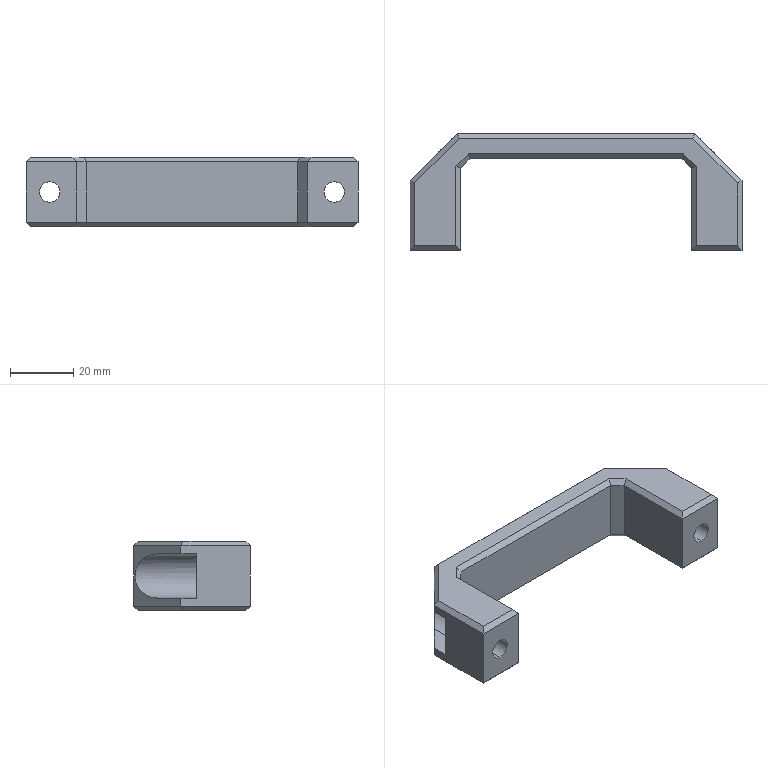Part | SolidWorks | features Chamfer 1, Extrusion 1, HoleWzd 1, ICE 1 | 1 solid | 56 faces | box 105 x 37 x 22 mm | volume 26847 mm3 | plane 46 | cylinder 10 | commonest cylinder face diameters 6.5 x4 11 x4 14 x2
STEP:
#1=CARTESIAN_POINT('',(-45.,0.,-3.25));
#2=VERTEX_POINT('',#1);
#3=CARTESIAN_POINT('',(-45.,0.,3.25));
#4=VERTEX_POINT('',#3);
#5=CARTESIAN_POINT('',(-45.,0.,0.));
#6=DIRECTION('',(0.,1.,0.));
#7=DIRECTION('',(0.,0.,1.));
#8=AXIS2_PLACEMENT_3D('',#5,#6,#7);
#9=CIRCLE('',#8,3.25);
#10=EDGE_CURVE('',#2,#4,#9,.T.);
#11=ORIENTED_EDGE('',*,*,#10,.F.);
#12=CARTESIAN_POINT('',(-45.,7.,-3.25));
#13=VERTEX_POINT('',#12);
#14=CARTESIAN_POINT('',(-45.,37.,-3.25));
#15=DIRECTION('',(0.,1.,0.));
#16=VECTOR('',#15,1000.);
#17=LINE('',#14,#16);
#18=EDGE_CURVE('',#2,#13,#17,.T.);
#19=ORIENTED_EDGE('',*,*,#18,.T.);
#20=CARTESIAN_POINT('',(-45.,7.,3.25));
#21=VERTEX_POINT('',#20);
#22=CARTESIAN_POINT('',(-45.,7.,0.));
#23=DIRECTION('',(0.,1.,0.));
#24=DIRECTION('',(0.,0.,1.));
#25=AXIS2_PLACEMENT_3D('',#22,#23,#24);
#26=CIRCLE('',#25,3.25);
#27=EDGE_CURVE('',#13,#21,#26,.T.);
#28=ORIENTED_EDGE('',*,*,#27,.T.);
#29=CARTESIAN_POINT('',(-45.,37.,3.25));
#30=DIRECTION('',(0.,1.,0.));
#31=VECTOR('',#30,1000.);
#32=LINE('',#29,#31);
#33=EDGE_CURVE('',#4,#21,#32,.T.);
#34=ORIENTED_EDGE('',*,*,#33,.F.);
#35=EDGE_LOOP('',(#11,#19,#28,#34));
#36=FACE_OUTER_BOUND('',#35,.T.);
#37=CARTESIAN_POINT('',(-45.,37.,0.));
#38=DIRECTION('',(0.,1.,0.));
#39=DIRECTION('',(0.,0.,1.));
#40=AXIS2_PLACEMENT_3D('',#37,#38,#39);
#41=CYLINDRICAL_SURFACE('',#40,3.25);
#42=ADVANCED_FACE('',(#36),#41,.F.);
#43=CARTESIAN_POINT('',(45.,0.,-3.25));
#44=VERTEX_POINT('',#43);
#45=CARTESIAN_POINT('',(45.,0.,3.25));
#46=VERTEX_POINT('',#45);
#47=CARTESIAN_POINT('',(45.,0.,0.));
#48=DIRECTION('',(0.,1.,0.));
#49=DIRECTION('',(0.,0.,1.));
#50=AXIS2_PLACEMENT_3D('',#47,#48,#49);
#51=CIRCLE('',#50,3.25);
#52=EDGE_CURVE('',#44,#46,#51,.T.);
#53=ORIENTED_EDGE('',*,*,#52,.F.);
#54=CARTESIAN_POINT('',(45.,7.,-3.25));
#55=VERTEX_POINT('',#54);
#56=CARTESIAN_POINT('',(45.,37.,-3.25));
#57=DIRECTION('',(0.,1.,0.));
#58=VECTOR('',#57,1000.);
#59=LINE('',#56,#58);
#60=EDGE_CURVE('',#44,#55,#59,.T.);
#61=ORIENTED_EDGE('',*,*,#60,.T.);
#62=CARTESIAN_POINT('',(45.,7.,3.25));
#63=VERTEX_POINT('',#62);
#64=CARTESIAN_POINT('',(45.,7.,0.));
#65=DIRECTION('',(0.,1.,0.));
#66=DIRECTION('',(0.,0.,1.));
#67=AXIS2_PLACEMENT_3D('',#64,#65,#66);
#68=CIRCLE('',#67,3.25);
#69=EDGE_CURVE('',#55,#63,#68,.T.);
#70=ORIENTED_EDGE('',*,*,#69,.T.);
#71=CARTESIAN_POINT('',(45.,37.,3.25));
#72=DIRECTION('',(0.,1.,0.));
#73=VECTOR('',#72,1000.);
#74=LINE('',#71,#73);
#75=EDGE_CURVE('',#46,#63,#74,.T.);
#76=ORIENTED_EDGE('',*,*,#75,.F.);
#77=EDGE_LOOP('',(#53,#61,#70,#76));
#78=FACE_OUTER_BOUND('',#77,.T.);
#79=CARTESIAN_POINT('',(45.,37.,0.));
#80=DIRECTION('',(0.,1.,0.));
#81=DIRECTION('',(0.,0.,1.));
#82=AXIS2_PLACEMENT_3D('',#79,#80,#81);
#83=CYLINDRICAL_SURFACE('',#82,3.25);
#84=ADVANCED_FACE('',(#78),#83,.F.);
#85=CARTESIAN_POINT('',(45.,7.,-5.5));
#86=VERTEX_POINT('',#85);
#87=CARTESIAN_POINT('',(45.,7.,5.5));
#88=VERTEX_POINT('',#87);
#89=CARTESIAN_POINT('',(45.,7.,0.));
#90=DIRECTION('',(0.,1.,0.));
#91=DIRECTION('',(0.,0.,1.));
#92=AXIS2_PLACEMENT_3D('',#89,#90,#91);
#93=CIRCLE('',#92,5.5);
#94=EDGE_CURVE('',#86,#88,#93,.T.);
#95=ORIENTED_EDGE('',*,*,#94,.F.);
#96=CARTESIAN_POINT('',(45.,17.,-5.5));
#97=VERTEX_POINT('',#96);
#98=CARTESIAN_POINT('',(45.,37.,-5.5));
#99=DIRECTION('',(0.,1.,0.));
#100=VECTOR('',#99,1000.);
#101=LINE('',#98,#100);
#102=EDGE_CURVE('',#86,#97,#101,.T.);
#103=ORIENTED_EDGE('',*,*,#102,.T.);
#104=CARTESIAN_POINT('',(45.,17.,5.5));
#105=VERTEX_POINT('',#104);
#106=CARTESIAN_POINT('',(45.,17.,0.));
#107=DIRECTION('',(0.,1.,0.));
#108=DIRECTION('',(0.,0.,-1.));
#109=AXIS2_PLACEMENT_3D('',#106,#107,#108);
#110=CIRCLE('',#109,5.5);
#111=EDGE_CURVE('',#97,#105,#110,.T.);
#112=ORIENTED_EDGE('',*,*,#111,.T.);
#113=CARTESIAN_POINT('',(45.,37.,5.5));
#114=DIRECTION('',(0.,1.,0.));
#115=VECTOR('',#114,1000.);
#116=LINE('',#113,#115);
#117=EDGE_CURVE('',#88,#105,#116,.T.);
#118=ORIENTED_EDGE('',*,*,#117,.F.);
#119=EDGE_LOOP('',(#95,#103,#112,#118));
#120=FACE_OUTER_BOUND('',#119,.T.);
#121=CARTESIAN_POINT('',(45.,37.,0.));
#122=DIRECTION('',(0.,1.,0.));
#123=DIRECTION('',(0.,0.,1.));
#124=AXIS2_PLACEMENT_3D('',#121,#122,#123);
#125=CYLINDRICAL_SURFACE('',#124,5.5);
#126=ADVANCED_FACE('',(#120),#125,.F.);
#127=CARTESIAN_POINT('',(-45.,7.,-5.5));
#128=VERTEX_POINT('',#127);
#129=CARTESIAN_POINT('',(-45.,7.,5.5));
#130=VERTEX_POINT('',#129);
#131=CARTESIAN_POINT('',(-45.,7.,0.));
#132=DIRECTION('',(0.,1.,0.));
#133=DIRECTION('',(0.,0.,1.));
#134=AXIS2_PLACEMENT_3D('',#131,#132,#133);
#135=CIRCLE('',#134,5.5);
#136=EDGE_CURVE('',#128,#130,#135,.T.);
#137=ORIENTED_EDGE('',*,*,#136,.F.);
#138=CARTESIAN_POINT('',(-45.,17.,-5.5));
#139=VERTEX_POINT('',#138);
#140=CARTESIAN_POINT('',(-45.,37.,-5.5));
#141=DIRECTION('',(0.,1.,0.));
#142=VECTOR('',#141,1000.);
#143=LINE('',#140,#142);
#144=EDGE_CURVE('',#128,#139,#143,.T.);
#145=ORIENTED_EDGE('',*,*,#144,.T.);
#146=CARTESIAN_POINT('',(-45.,17.,5.5));
#147=VERTEX_POINT('',#146);
#148=CARTESIAN_POINT('',(-45.,17.,0.));
#149=DIRECTION('',(0.,-1.,0.));
#150=DIRECTION('',(0.,0.,1.));
#151=AXIS2_PLACEMENT_3D('',#148,#149,#150);
#152=CIRCLE('',#151,5.5);
#153=EDGE_CURVE('',#147,#139,#152,.T.);
#154=ORIENTED_EDGE('',*,*,#153,.F.);
#155=CARTESIAN_POINT('',(-45.,37.,5.5));
#156=DIRECTION('',(0.,1.,0.));
#157=VECTOR('',#156,1000.);
#158=LINE('',#155,#157);
#159=EDGE_CURVE('',#130,#147,#158,.T.);
#160=ORIENTED_EDGE('',*,*,#159,.F.);
#161=EDGE_LOOP('',(#137,#145,#154,#160));
#162=FACE_OUTER_BOUND('',#161,.T.);
#163=CARTESIAN_POINT('',(-45.,37.,0.));
#164=DIRECTION('',(0.,1.,0.));
#165=DIRECTION('',(0.,0.,1.));
#166=AXIS2_PLACEMENT_3D('',#163,#164,#165);
#167=CYLINDRICAL_SURFACE('',#166,5.5);
#168=ADVANCED_FACE('',(#162),#167,.F.);
#169=ORIENTED_EDGE('',*,*,#144,.F.);
#170=CARTESIAN_POINT('',(-45.,7.,0.));
#171=DIRECTION('',(0.,1.,0.));
#172=DIRECTION('',(0.,0.,1.));
#173=AXIS2_PLACEMENT_3D('',#170,#171,#172);
#174=CIRCLE('',#173,5.5);
#175=EDGE_CURVE('',#130,#128,#174,.T.);
#176=ORIENTED_EDGE('',*,*,#175,.F.);
#177=ORIENTED_EDGE('',*,*,#159,.T.);
#178=CARTESIAN_POINT('',(-45.,17.,0.));
#179=DIRECTION('',(0.,-1.,0.));
#180=DIRECTION('',(0.,0.,1.));
#181=AXIS2_PLACEMENT_3D('',#178,#179,#180);
#182=CIRCLE('',#181,5.5);
#183=EDGE_CURVE('',#139,#147,#182,.T.);
#184=ORIENTED_EDGE('',*,*,#183,.F.);
#185=EDGE_LOOP('',(#169,#176,#177,#184));
#186=FACE_OUTER_BOUND('',#185,.T.);
#187=CARTESIAN_POINT('',(-45.,37.,0.));
#188=DIRECTION('',(0.,1.,0.));
#189=DIRECTION('',(0.,0.,1.));
#190=AXIS2_PLACEMENT_3D('',#187,#188,#189);
#191=CYLINDRICAL_SURFACE('',#190,5.5);
#192=ADVANCED_FACE('',(#186),#191,.F.);
#193=CARTESIAN_POINT('',(-52.5,22.,-7.));
#194=VERTEX_POINT('',#193);
#195=CARTESIAN_POINT('',(-52.5,22.,-9.5));
#196=VERTEX_POINT('',#195);
#197=CARTESIAN_POINT('',(-52.5,22.,11.));
#198=DIRECTION('',(0.,0.,-1.));
#199=VECTOR('',#198,1000.);
#200=LINE('',#197,#199);
#201=EDGE_CURVE('',#194,#196,#200,.T.);
#202=ORIENTED_EDGE('',*,*,#201,.T.);
#203=CARTESIAN_POINT('',(-52.5,0.,-9.5));
#204=VERTEX_POINT('',#203);
#205=CARTESIAN_POINT('',(-52.5,22.,-9.5));
#206=DIRECTION('',(0.,-1.,0.));
#207=VECTOR('',#206,1000.);
#208=LINE('',#205,#207);
#209=EDGE_CURVE('',#196,#204,#208,.T.);
#210=ORIENTED_EDGE('',*,*,#209,.T.);
#211=CARTESIAN_POINT('',(-52.5,0.,9.5));
#212=VERTEX_POINT('',#211);
#213=CARTESIAN_POINT('',(-52.5,0.,11.));
#214=DIRECTION('',(0.,0.,-1.));
#215=VECTOR('',#214,1000.);
#216=LINE('',#213,#215);
#217=EDGE_CURVE('',#212,#204,#216,.T.);
#218=ORIENTED_EDGE('',*,*,#217,.F.);
#219=CARTESIAN_POINT('',(-52.5,22.,9.5));
#220=VERTEX_POINT('',#219);
#221=CARTESIAN_POINT('',(-52.5,22.,9.5));
#222=DIRECTION('',(0.,1.,0.));
#223=VECTOR('',#222,1000.);
#224=LINE('',#221,#223);
#225=EDGE_CURVE('',#212,#220,#224,.T.);
#226=ORIENTED_EDGE('',*,*,#225,.T.);
#227=CARTESIAN_POINT('',(-52.5,22.,7.));
#228=VERTEX_POINT('',#227);
#229=CARTESIAN_POINT('',(-52.5,22.,11.));
#230=DIRECTION('',(0.,0.,-1.));
#231=VECTOR('',#230,1000.);
#232=LINE('',#229,#231);
#233=EDGE_CURVE('',#220,#228,#232,.T.);
#234=ORIENTED_EDGE('',*,*,#233,.T.);
#235=CARTESIAN_POINT('',(-52.5,17.,7.));
#236=VERTEX_POINT('',#235);
#237=CARTESIAN_POINT('',(-52.5,17.,7.));
#238=DIRECTION('',(0.,1.,0.));
#239=VECTOR('',#238,1000.);
#240=LINE('',#237,#239);
#241=EDGE_CURVE('',#236,#228,#240,.T.);
#242=ORIENTED_EDGE('',*,*,#241,.F.);
#243=CARTESIAN_POINT('',(-52.5,17.,-7.));
#244=VERTEX_POINT('',#243);
#245=CARTESIAN_POINT('',(-52.5,17.,11.));
#246=DIRECTION('',(0.,0.,1.));
#247=VECTOR('',#246,1000.);
#248=LINE('',#245,#247);
#249=EDGE_CURVE('',#244,#236,#248,.T.);
#250=ORIENTED_EDGE('',*,*,#249,.F.);
#251=CARTESIAN_POINT('',(-52.5,17.,-7.));
#252=DIRECTION('',(0.,1.,0.));
#253=VECTOR('',#252,1000.);
#254=LINE('',#251,#253);
#255=EDGE_CURVE('',#244,#194,#254,.T.);
#256=ORIENTED_EDGE('',*,*,#255,.T.);
#257=EDGE_LOOP('',(#202,#210,#218,#226,#234,#242,#250,#256));
#258=FACE_OUTER_BOUND('',#257,.T.);
#259=CARTESIAN_POINT('',(-52.5,22.,11.));
#260=DIRECTION('',(1.,0.,0.));
#261=DIRECTION('',(0.,1.,0.));
#262=AXIS2_PLACEMENT_3D('',#259,#260,#261);
#263=PLANE('',#262);
#264=ADVANCED_FACE('',(#258),#263,.F.);
#265=CARTESIAN_POINT('',(-45.,0.,0.));
#266=DIRECTION('',(0.,1.,0.));
#267=DIRECTION('',(0.,0.,1.));
#268=AXIS2_PLACEMENT_3D('',#265,#266,#267);
#269=CIRCLE('',#268,3.25);
#270=EDGE_CURVE('',#4,#2,#269,.T.);
#271=ORIENTED_EDGE('',*,*,#270,.T.);
#272=ORIENTED_EDGE('',*,*,#10,.T.);
#273=EDGE_LOOP('',(#271,#272));
#274=FACE_BOUND('',#273,.T.);
#275=ORIENTED_EDGE('',*,*,#217,.T.);
#276=CARTESIAN_POINT('',(-36.5,0.,-9.5));
#277=VERTEX_POINT('',#276);
#278=CARTESIAN_POINT('',(-52.5,0.,-9.5));
#279=DIRECTION('',(1.,0.,0.));
#280=VECTOR('',#279,1000.);
#281=LINE('',#278,#280);
#282=EDGE_CURVE('',#204,#277,#281,.T.);
#283=ORIENTED_EDGE('',*,*,#282,.T.);
#284=CARTESIAN_POINT('',(-36.5,0.,9.5));
#285=VERTEX_POINT('',#284);
#286=CARTESIAN_POINT('',(-36.5,0.,11.));
#287=DIRECTION('',(0.,0.,-1.));
#288=VECTOR('',#287,1000.);
#289=LINE('',#286,#288);
#290=EDGE_CURVE('',#285,#277,#289,.T.);
#291=ORIENTED_EDGE('',*,*,#290,.F.);
#292=CARTESIAN_POINT('',(-52.5,0.,9.5));
#293=DIRECTION('',(-1.,0.,0.));
#294=VECTOR('',#293,1000.);
#295=LINE('',#292,#294);
#296=EDGE_CURVE('',#285,#212,#295,.T.);
#297=ORIENTED_EDGE('',*,*,#296,.T.);
#298=EDGE_LOOP('',(#275,#283,#291,#297));
#299=FACE_OUTER_BOUND('',#298,.T.);
#300=CARTESIAN_POINT('',(-52.5,0.,11.));
#301=DIRECTION('',(0.,1.,0.));
#302=DIRECTION('',(0.,0.,1.));
#303=AXIS2_PLACEMENT_3D('',#300,#301,#302);
#304=PLANE('',#303);
#305=ADVANCED_FACE('',(#274,#299),#304,.F.);
#306=ORIENTED_EDGE('',*,*,#290,.T.);
#307=CARTESIAN_POINT('',(-36.5,26.,-9.5));
#308=VERTEX_POINT('',#307);
#309=CARTESIAN_POINT('',(-36.5,0.,-9.5));
#310=DIRECTION('',(0.,1.,0.));
#311=VECTOR('',#310,1000.);
#312=LINE('',#309,#311);
#313=EDGE_CURVE('',#277,#308,#312,.T.);
#314=ORIENTED_EDGE('',*,*,#313,.T.);
#315=CARTESIAN_POINT('',(-36.5,26.,9.5));
#316=VERTEX_POINT('',#315);
#317=CARTESIAN_POINT('',(-36.5,26.,11.));
#318=DIRECTION('',(0.,0.,-1.));
#319=VECTOR('',#318,1000.);
#320=LINE('',#317,#319);
#321=EDGE_CURVE('',#316,#308,#320,.T.);
#322=ORIENTED_EDGE('',*,*,#321,.F.);
#323=CARTESIAN_POINT('',(-36.5,0.,9.5));
#324=DIRECTION('',(0.,-1.,0.));
#325=VECTOR('',#324,1000.);
#326=LINE('',#323,#325);
#327=EDGE_CURVE('',#316,#285,#326,.T.);
#328=ORIENTED_EDGE('',*,*,#327,.T.);
#329=EDGE_LOOP('',(#306,#314,#322,#328));
#330=FACE_OUTER_BOUND('',#329,.T.);
#331=CARTESIAN_POINT('',(-36.5,0.,11.));
#332=DIRECTION('',(-1.,0.,0.));
#333=DIRECTION('',(0.,0.,1.));
#334=AXIS2_PLACEMENT_3D('',#331,#332,#333);
#335=PLANE('',#334);
#336=ADVANCED_FACE('',(#330),#335,.F.);
#337=ORIENTED_EDGE('',*,*,#321,.T.);
#338=CARTESIAN_POINT('',(-33.5,29.,-9.5));
#339=VERTEX_POINT('',#338);
#340=CARTESIAN_POINT('',(-36.5,26.,-9.5));
#341=DIRECTION('',(0.7071,0.7071,0.));
#342=VECTOR('',#341,1000.);
#343=LINE('',#340,#342);
#344=EDGE_CURVE('',#308,#339,#343,.T.);
#345=ORIENTED_EDGE('',*,*,#344,.T.);
#346=CARTESIAN_POINT('',(-33.5,29.,9.5));
#347=VERTEX_POINT('',#346);
#348=CARTESIAN_POINT('',(-33.5,29.,11.));
#349=DIRECTION('',(0.,0.,-1.));
#350=VECTOR('',#349,1000.);
#351=LINE('',#348,#350);
#352=EDGE_CURVE('',#347,#339,#351,.T.);
#353=ORIENTED_EDGE('',*,*,#352,.F.);
#354=CARTESIAN_POINT('',(-36.5,26.,9.5));
#355=DIRECTION('',(-0.7071,-0.7071,0.));
#356=VECTOR('',#355,1000.);
#357=LINE('',#354,#356);
#358=EDGE_CURVE('',#347,#316,#357,.T.);
#359=ORIENTED_EDGE('',*,*,#358,.T.);
#360=EDGE_LOOP('',(#337,#345,#353,#359));
#361=FACE_OUTER_BOUND('',#360,.T.);
#362=CARTESIAN_POINT('',(-36.5,26.,11.));
#363=DIRECTION('',(-0.7071,0.7071,0.));
#364=DIRECTION('',(-0.7071,-0.7071,0.));
#365=AXIS2_PLACEMENT_3D('',#362,#363,#364);
#366=PLANE('',#365);
#367=ADVANCED_FACE('',(#361),#366,.F.);
#368=ORIENTED_EDGE('',*,*,#352,.T.);
#369=CARTESIAN_POINT('',(33.5,29.,-9.5));
#370=VERTEX_POINT('',#369);
#371=CARTESIAN_POINT('',(-33.5,29.,-9.5));
#372=DIRECTION('',(1.,0.,0.));
#373=VECTOR('',#372,1000.);
#374=LINE('',#371,#373);
#375=EDGE_CURVE('',#339,#370,#374,.T.);
#376=ORIENTED_EDGE('',*,*,#375,.T.);
#377=CARTESIAN_POINT('',(33.5,29.,9.5));
#378=VERTEX_POINT('',#377);
#379=CARTESIAN_POINT('',(33.5,29.,11.));
#380=DIRECTION('',(0.,0.,-1.));
#381=VECTOR('',#380,1000.);
#382=LINE('',#379,#381);
#383=EDGE_CURVE('',#378,#370,#382,.T.);
#384=ORIENTED_EDGE('',*,*,#383,.F.);
#385=CARTESIAN_POINT('',(-33.5,29.,9.5));
#386=DIRECTION('',(-1.,0.,0.));
#387=VECTOR('',#386,1000.);
#388=LINE('',#385,#387);
#389=EDGE_CURVE('',#378,#347,#388,.T.);
#390=ORIENTED_EDGE('',*,*,#389,.T.);
#391=EDGE_LOOP('',(#368,#376,#384,#390));
#392=FACE_OUTER_BOUND('',#391,.T.);
#393=CARTESIAN_POINT('',(-33.5,29.,11.));
#394=DIRECTION('',(0.,1.,0.));
#395=DIRECTION('',(0.,0.,1.));
#396=AXIS2_PLACEMENT_3D('',#393,#394,#395);
#397=PLANE('',#396);
#398=ADVANCED_FACE('',(#392),#397,.F.);
#399=ORIENTED_EDGE('',*,*,#383,.T.);
#400=CARTESIAN_POINT('',(36.5,26.,-9.5));
#401=VERTEX_POINT('',#400);
#402=CARTESIAN_POINT('',(33.5,29.,-9.5));
#403=DIRECTION('',(0.7071,-0.7071,0.));
#404=VECTOR('',#403,1000.);
#405=LINE('',#402,#404);
#406=EDGE_CURVE('',#370,#401,#405,.T.);
#407=ORIENTED_EDGE('',*,*,#406,.T.);
#408=CARTESIAN_POINT('',(36.5,26.,9.5));
#409=VERTEX_POINT('',#408);
#410=CARTESIAN_POINT('',(36.5,26.,11.));
#411=DIRECTION('',(0.,0.,-1.));
#412=VECTOR('',#411,1000.);
#413=LINE('',#410,#412);
#414=EDGE_CURVE('',#409,#401,#413,.T.);
#415=ORIENTED_EDGE('',*,*,#414,.F.);
#416=CARTESIAN_POINT('',(33.5,29.,9.5));
#417=DIRECTION('',(-0.7071,0.7071,0.));
#418=VECTOR('',#417,1000.);
#419=LINE('',#416,#418);
#420=EDGE_CURVE('',#409,#378,#419,.T.);
#421=ORIENTED_EDGE('',*,*,#420,.T.);
#422=EDGE_LOOP('',(#399,#407,#415,#421));
#423=FACE_OUTER_BOUND('',#422,.T.);
#424=CARTESIAN_POINT('',(33.5,29.,11.));
#425=DIRECTION('',(0.7071,0.7071,0.));
#426=DIRECTION('',(-0.7071,0.7071,0.));
#427=AXIS2_PLACEMENT_3D('',#424,#425,#426);
#428=PLANE('',#427);
#429=ADVANCED_FACE('',(#423),#428,.F.);
#430=ORIENTED_EDGE('',*,*,#414,.T.);
#431=CARTESIAN_POINT('',(36.5,0.,-9.5));
#432=VERTEX_POINT('',#431);
#433=CARTESIAN_POINT('',(36.5,26.,-9.5));
#434=DIRECTION('',(0.,-1.,0.));
#435=VECTOR('',#434,1000.);
#436=LINE('',#433,#435);
#437=EDGE_CURVE('',#401,#432,#436,.T.);
#438=ORIENTED_EDGE('',*,*,#437,.T.);
#439=CARTESIAN_POINT('',(36.5,0.,9.5));
#440=VERTEX_POINT('',#439);
#441=CARTESIAN_POINT('',(36.5,0.,11.));
#442=DIRECTION('',(0.,0.,-1.));
#443=VECTOR('',#442,1000.);
#444=LINE('',#441,#443);
#445=EDGE_CURVE('',#440,#432,#444,.T.);
#446=ORIENTED_EDGE('',*,*,#445,.F.);
#447=CARTESIAN_POINT('',(36.5,26.,9.5));
#448=DIRECTION('',(0.,1.,0.));
#449=VECTOR('',#448,1000.);
#450=LINE('',#447,#449);
#451=EDGE_CURVE('',#440,#409,#450,.T.);
#452=ORIENTED_EDGE('',*,*,#451,.T.);
#453=EDGE_LOOP('',(#430,#438,#446,#452));
#454=FACE_OUTER_BOUND('',#453,.T.);
#455=CARTESIAN_POINT('',(36.5,26.,11.));
#456=DIRECTION('',(1.,0.,0.));
#457=DIRECTION('',(0.,0.,-1.));
#458=AXIS2_PLACEMENT_3D('',#455,#456,#457);
#459=PLANE('',#458);
#460=ADVANCED_FACE('',(#454),#459,.F.);
#461=CARTESIAN_POINT('',(45.,0.,0.));
#462=DIRECTION('',(0.,1.,0.));
#463=DIRECTION('',(0.,0.,1.));
#464=AXIS2_PLACEMENT_3D('',#461,#462,#463);
#465=CIRCLE('',#464,3.25);
#466=EDGE_CURVE('',#46,#44,#465,.T.);
#467=ORIENTED_EDGE('',*,*,#466,.T.);
#468=ORIENTED_EDGE('',*,*,#52,.T.);
#469=EDGE_LOOP('',(#467,#468));
#470=FACE_BOUND('',#469,.T.);
#471=ORIENTED_EDGE('',*,*,#445,.T.);
#472=CARTESIAN_POINT('',(52.5,0.,-9.5));
#473=VERTEX_POINT('',#472);
#474=CARTESIAN_POINT('',(36.5,0.,-9.5));
#475=DIRECTION('',(1.,0.,0.));
#476=VECTOR('',#475,1000.);
#477=LINE('',#474,#476);
#478=EDGE_CURVE('',#432,#473,#477,.T.);
#479=ORIENTED_EDGE('',*,*,#478,.T.);
#480=CARTESIAN_POINT('',(52.5,0.,9.5));
#481=VERTEX_POINT('',#480);
#482=CARTESIAN_POINT('',(52.5,0.,11.));
#483=DIRECTION('',(0.,0.,-1.));
#484=VECTOR('',#483,1000.);
#485=LINE('',#482,#484);
#486=EDGE_CURVE('',#481,#473,#485,.T.);
#487=ORIENTED_EDGE('',*,*,#486,.F.);
#488=CARTESIAN_POINT('',(36.5,0.,9.5));
#489=DIRECTION('',(-1.,0.,0.));
#490=VECTOR('',#489,1000.);
#491=LINE('',#488,#490);
#492=EDGE_CURVE('',#481,#440,#491,.T.);
#493=ORIENTED_EDGE('',*,*,#492,.T.);
#494=EDGE_LOOP('',(#471,#479,#487,#493));
#495=FACE_OUTER_BOUND('',#494,.T.);
#496=CARTESIAN_POINT('',(36.5,0.,11.));
#497=DIRECTION('',(0.,1.,0.));
#498=DIRECTION('',(0.,0.,1.));
#499=AXIS2_PLACEMENT_3D('',#496,#497,#498);
#500=PLANE('',#499);
#501=ADVANCED_FACE('',(#470,#495),#500,.F.);
#502=ORIENTED_EDGE('',*,*,#486,.T.);
#503=CARTESIAN_POINT('',(52.5,22.,-9.5));
#504=VERTEX_POINT('',#503);
#505=CARTESIAN_POINT('',(52.5,0.,-9.5));
#506=DIRECTION('',(0.,1.,0.));
#507=VECTOR('',#506,1000.);
#508=LINE('',#505,#507);
#509=EDGE_CURVE('',#473,#504,#508,.T.);
#510=ORIENTED_EDGE('',*,*,#509,.T.);
#511=CARTESIAN_POINT('',(52.5,22.,-7.));
#512=VERTEX_POINT('',#511);
#513=CARTESIAN_POINT('',(52.5,22.,11.));
#514=DIRECTION('',(0.,0.,-1.));
#515=VECTOR('',#514,1000.);
#516=LINE('',#513,#515);
#517=EDGE_CURVE('',#512,#504,#516,.T.);
#518=ORIENTED_EDGE('',*,*,#517,.F.);
#519=CARTESIAN_POINT('',(52.5,17.,-7.));
#520=VERTEX_POINT('',#519);
#521=CARTESIAN_POINT('',(52.5,17.,-7.));
#522=DIRECTION('',(0.,1.,0.));
#523=VECTOR('',#522,1000.);
#524=LINE('',#521,#523);
#525=EDGE_CURVE('',#520,#512,#524,.T.);
#526=ORIENTED_EDGE('',*,*,#525,.F.);
#527=CARTESIAN_POINT('',(52.5,17.,7.));
#528=VERTEX_POINT('',#527);
#529=CARTESIAN_POINT('',(52.5,17.,11.));
#530=DIRECTION('',(0.,0.,1.));
#531=VECTOR('',#530,1000.);
#532=LINE('',#529,#531);
#533=EDGE_CURVE('',#520,#528,#532,.T.);
#534=ORIENTED_EDGE('',*,*,#533,.T.);
#535=CARTESIAN_POINT('',(52.5,22.,7.));
#536=VERTEX_POINT('',#535);
#537=CARTESIAN_POINT('',(52.5,17.,7.));
#538=DIRECTION('',(0.,1.,0.));
#539=VECTOR('',#538,1000.);
#540=LINE('',#537,#539);
#541=EDGE_CURVE('',#528,#536,#540,.T.);
#542=ORIENTED_EDGE('',*,*,#541,.T.);
#543=CARTESIAN_POINT('',(52.5,22.,9.5));
#544=VERTEX_POINT('',#543);
#545=CARTESIAN_POINT('',(52.5,22.,11.));
#546=DIRECTION('',(0.,0.,-1.));
#547=VECTOR('',#546,1000.);
#548=LINE('',#545,#547);
#549=EDGE_CURVE('',#544,#536,#548,.T.);
#550=ORIENTED_EDGE('',*,*,#549,.F.);
#551=CARTESIAN_POINT('',(52.5,0.,9.5));
#552=DIRECTION('',(0.,-1.,0.));
#553=VECTOR('',#552,1000.);
#554=LINE('',#551,#553);
#555=EDGE_CURVE('',#544,#481,#554,.T.);
#556=ORIENTED_EDGE('',*,*,#555,.T.);
#557=EDGE_LOOP('',(#502,#510,#518,#526,#534,#542,#550,#556));
#558=FACE_OUTER_BOUND('',#557,.T.);
#559=CARTESIAN_POINT('',(52.5,0.,11.));
#560=DIRECTION('',(-1.,0.,0.));
#561=DIRECTION('',(0.,-1.,0.));
#562=AXIS2_PLACEMENT_3D('',#559,#560,#561);
#563=PLANE('',#562);
#564=ADVANCED_FACE('',(#558),#563,.F.);
#565=ORIENTED_EDGE('',*,*,#517,.T.);
#566=CARTESIAN_POINT('',(37.5,37.,-9.5));
#567=VERTEX_POINT('',#566);
#568=CARTESIAN_POINT('',(52.5,22.,-9.5));
#569=DIRECTION('',(-0.7071,0.7071,0.));
#570=VECTOR('',#569,1000.);
#571=LINE('',#568,#570);
#572=EDGE_CURVE('',#504,#567,#571,.T.);
#573=ORIENTED_EDGE('',*,*,#572,.T.);
#574=CARTESIAN_POINT('',(37.5,37.,9.5));
#575=VERTEX_POINT('',#574);
#576=CARTESIAN_POINT('',(37.5,37.,11.));
#577=DIRECTION('',(0.,0.,-1.));
#578=VECTOR('',#577,1000.);
#579=LINE('',#576,#578);
#580=EDGE_CURVE('',#575,#567,#579,.T.);
#581=ORIENTED_EDGE('',*,*,#580,.F.);
#582=CARTESIAN_POINT('',(52.5,22.,9.5));
#583=DIRECTION('',(0.7071,-0.7071,0.));
#584=VECTOR('',#583,1000.);
#585=LINE('',#582,#584);
#586=EDGE_CURVE('',#575,#544,#585,.T.);
#587=ORIENTED_EDGE('',*,*,#586,.T.);
#588=ORIENTED_EDGE('',*,*,#549,.T.);
#589=CARTESIAN_POINT('',(45.,29.5,7.));
#590=VERTEX_POINT('',#589);
#591=CARTESIAN_POINT('',(52.5,22.,7.));
#592=DIRECTION('',(-0.7071,0.7071,0.));
#593=VECTOR('',#592,1000.);
#594=LINE('',#591,#593);
#595=EDGE_CURVE('',#536,#590,#594,.T.);
#596=ORIENTED_EDGE('',*,*,#595,.T.);
#597=CARTESIAN_POINT('',(45.,29.5,-7.));
#598=VERTEX_POINT('',#597);
#599=CARTESIAN_POINT('',(45.,29.5,7.));
#600=CARTESIAN_POINT('',(31.,43.5,7.));
#601=CARTESIAN_POINT('',(31.,43.5,-7.));
#602=CARTESIAN_POINT('',(45.,29.5,-7.));
#603=(BOUNDED_CURVE()B_SPLINE_CURVE(3,(#599,#600,#601,#602),.UNSPECIFIED.,.F.,.F.)B_SPLINE_CURVE_WITH_KNOTS((4,4),(4.712,7.854),.UNSPECIFIED.)CURVE()GEOMETRIC_REPRESENTATION_ITEM()RATIONAL_B_SPLINE_CURVE((1.,0.3333,0.3333,1.))REPRESENTATION_ITEM(''));
#604=EDGE_CURVE('',#590,#598,#603,.T.);
#605=ORIENTED_EDGE('',*,*,#604,.T.);
#606=CARTESIAN_POINT('',(52.5,22.,-7.));
#607=DIRECTION('',(0.7071,-0.7071,0.));
#608=VECTOR('',#607,1000.);
#609=LINE('',#606,#608);
#610=EDGE_CURVE('',#598,#512,#609,.T.);
#611=ORIENTED_EDGE('',*,*,#610,.T.);
#612=EDGE_LOOP('',(#565,#573,#581,#587,#588,#596,#605,#611));
#613=FACE_OUTER_BOUND('',#612,.T.);
#614=CARTESIAN_POINT('',(52.5,22.,11.));
#615=DIRECTION('',(-0.7071,-0.7071,0.));
#616=DIRECTION('',(0.7071,-0.7071,0.));
#617=AXIS2_PLACEMENT_3D('',#614,#615,#616);
#618=PLANE('',#617);
#619=ADVANCED_FACE('',(#613),#618,.F.);
#620=ORIENTED_EDGE('',*,*,#580,.T.);
#621=CARTESIAN_POINT('',(-37.5,37.,-9.5));
#622=VERTEX_POINT('',#621);
#623=CARTESIAN_POINT('',(37.5,37.,-9.5));
#624=DIRECTION('',(-1.,0.,0.));
#625=VECTOR('',#624,1000.);
#626=LINE('',#623,#625);
#627=EDGE_CURVE('',#567,#622,#626,.T.);
#628=ORIENTED_EDGE('',*,*,#627,.T.);
#629=CARTESIAN_POINT('',(-37.5,37.,9.5));
#630=VERTEX_POINT('',#629);
#631=CARTESIAN_POINT('',(-37.5,37.,11.));
#632=DIRECTION('',(0.,0.,-1.));
#633=VECTOR('',#632,1000.);
#634=LINE('',#631,#633);
#635=EDGE_CURVE('',#630,#622,#634,.T.);
#636=ORIENTED_EDGE('',*,*,#635,.F.);
#637=CARTESIAN_POINT('',(37.5,37.,9.5));
#638=DIRECTION('',(1.,0.,0.));
#639=VECTOR('',#638,1000.);
#640=LINE('',#637,#639);
#641=EDGE_CURVE('',#630,#575,#640,.T.);
#642=ORIENTED_EDGE('',*,*,#641,.T.);
#643=EDGE_LOOP('',(#620,#628,#636,#642));
#644=FACE_OUTER_BOUND('',#643,.T.);
#645=CARTESIAN_POINT('',(37.5,37.,11.));
#646=DIRECTION('',(0.,-1.,0.));
#647=DIRECTION('',(0.,0.,-1.));
#648=AXIS2_PLACEMENT_3D('',#645,#646,#647);
#649=PLANE('',#648);
#650=ADVANCED_FACE('',(#644),#649,.F.);
#651=ORIENTED_EDGE('',*,*,#635,.T.);
#652=CARTESIAN_POINT('',(-37.5,37.,-9.5));
#653=DIRECTION('',(-0.7071,-0.7071,0.));
#654=VECTOR('',#653,1000.);
#655=LINE('',#652,#654);
#656=EDGE_CURVE('',#622,#196,#655,.T.);
#657=ORIENTED_EDGE('',*,*,#656,.T.);
#658=ORIENTED_EDGE('',*,*,#201,.F.);
#659=CARTESIAN_POINT('',(-45.,29.5,-7.));
#660=VERTEX_POINT('',#659);
#661=CARTESIAN_POINT('',(-37.5,37.,-7.));
#662=DIRECTION('',(0.7071,0.7071,0.));
#663=VECTOR('',#662,1000.);
#664=LINE('',#661,#663);
#665=EDGE_CURVE('',#194,#660,#664,.T.);
#666=ORIENTED_EDGE('',*,*,#665,.T.);
#667=CARTESIAN_POINT('',(-45.,29.5,7.));
#668=VERTEX_POINT('',#667);
#669=CARTESIAN_POINT('',(-45.,29.5,-7.));
#670=CARTESIAN_POINT('',(-31.,43.5,-7.));
#671=CARTESIAN_POINT('',(-31.,43.5,7.));
#672=CARTESIAN_POINT('',(-45.,29.5,7.));
#673=(BOUNDED_CURVE()B_SPLINE_CURVE(3,(#669,#670,#671,#672),.UNSPECIFIED.,.F.,.F.)B_SPLINE_CURVE_WITH_KNOTS((4,4),(4.712,7.854),.UNSPECIFIED.)CURVE()GEOMETRIC_REPRESENTATION_ITEM()RATIONAL_B_SPLINE_CURVE((1.,0.3333,0.3333,1.))REPRESENTATION_ITEM(''));
#674=EDGE_CURVE('',#660,#668,#673,.T.);
#675=ORIENTED_EDGE('',*,*,#674,.T.);
#676=CARTESIAN_POINT('',(-37.5,37.,7.));
#677=DIRECTION('',(-0.7071,-0.7071,0.));
#678=VECTOR('',#677,1000.);
#679=LINE('',#676,#678);
#680=EDGE_CURVE('',#668,#228,#679,.T.);
#681=ORIENTED_EDGE('',*,*,#680,.T.);
#682=ORIENTED_EDGE('',*,*,#233,.F.);
#683=CARTESIAN_POINT('',(-37.5,37.,9.5));
#684=DIRECTION('',(0.7071,0.7071,0.));
#685=VECTOR('',#684,1000.);
#686=LINE('',#683,#685);
#687=EDGE_CURVE('',#220,#630,#686,.T.);
#688=ORIENTED_EDGE('',*,*,#687,.T.);
#689=EDGE_LOOP('',(#651,#657,#658,#666,#675,#681,#682,#688));
#690=FACE_OUTER_BOUND('',#689,.T.);
#691=CARTESIAN_POINT('',(-37.5,37.,11.));
#692=DIRECTION('',(0.7071,-0.7071,0.));
#693=DIRECTION('',(0.7071,0.7071,0.));
#694=AXIS2_PLACEMENT_3D('',#691,#692,#693);
#695=PLANE('',#694);
#696=ADVANCED_FACE('',(#690),#695,.F.);
#697=CARTESIAN_POINT('',(36.879,35.5,11.));
#698=VERTEX_POINT('',#697);
#699=CARTESIAN_POINT('',(-36.879,35.5,11.));
#700=VERTEX_POINT('',#699);
#701=CARTESIAN_POINT('',(-37.5,35.5,11.));
#702=DIRECTION('',(-1.,0.,0.));
#703=VECTOR('',#702,1000.);
#704=LINE('',#701,#703);
#705=EDGE_CURVE('',#698,#700,#704,.T.);
#706=ORIENTED_EDGE('',*,*,#705,.T.);
#707=CARTESIAN_POINT('',(-51.,21.379,11.));
#708=VERTEX_POINT('',#707);
#709=CARTESIAN_POINT('',(-51.439,20.939,11.));
#710=DIRECTION('',(-0.7071,-0.7071,0.));
#711=VECTOR('',#710,1000.);
#712=LINE('',#709,#711);
#713=EDGE_CURVE('',#700,#708,#712,.T.);
#714=ORIENTED_EDGE('',*,*,#713,.T.);
#715=CARTESIAN_POINT('',(-51.,1.5,11.));
#716=VERTEX_POINT('',#715);
#717=CARTESIAN_POINT('',(-51.,0.,11.));
#718=DIRECTION('',(0.,-1.,0.));
#719=VECTOR('',#718,1000.);
#720=LINE('',#717,#719);
#721=EDGE_CURVE('',#708,#716,#720,.T.);
#722=ORIENTED_EDGE('',*,*,#721,.T.);
#723=CARTESIAN_POINT('',(-38.,1.5,11.));
#724=VERTEX_POINT('',#723);
#725=CARTESIAN_POINT('',(-36.5,1.5,11.));
#726=DIRECTION('',(1.,0.,0.));
#727=VECTOR('',#726,1000.);
#728=LINE('',#725,#727);
#729=EDGE_CURVE('',#716,#724,#728,.T.);
#730=ORIENTED_EDGE('',*,*,#729,.T.);
#731=CARTESIAN_POINT('',(-38.,26.621,11.));
#732=VERTEX_POINT('',#731);
#733=CARTESIAN_POINT('',(-38.,26.,11.));
#734=DIRECTION('',(0.,1.,0.));
#735=VECTOR('',#734,1000.);
#736=LINE('',#733,#735);
#737=EDGE_CURVE('',#724,#732,#736,.T.);
#738=ORIENTED_EDGE('',*,*,#737,.T.);
#739=CARTESIAN_POINT('',(-34.121,30.5,11.));
#740=VERTEX_POINT('',#739);
#741=CARTESIAN_POINT('',(-34.561,30.061,11.));
#742=DIRECTION('',(0.7071,0.7071,0.));
#743=VECTOR('',#742,1000.);
#744=LINE('',#741,#743);
#745=EDGE_CURVE('',#732,#740,#744,.T.);
#746=ORIENTED_EDGE('',*,*,#745,.T.);
#747=CARTESIAN_POINT('',(34.121,30.5,11.));
#748=VERTEX_POINT('',#747);
#749=CARTESIAN_POINT('',(33.5,30.5,11.));
#750=DIRECTION('',(1.,0.,0.));
#751=VECTOR('',#750,1000.);
#752=LINE('',#749,#751);
#753=EDGE_CURVE('',#740,#748,#752,.T.);
#754=ORIENTED_EDGE('',*,*,#753,.T.);
#755=CARTESIAN_POINT('',(38.,26.621,11.));
#756=VERTEX_POINT('',#755);
#757=CARTESIAN_POINT('',(37.561,27.061,11.));
#758=DIRECTION('',(0.7071,-0.7071,0.));
#759=VECTOR('',#758,1000.);
#760=LINE('',#757,#759);
#761=EDGE_CURVE('',#748,#756,#760,.T.);
#762=ORIENTED_EDGE('',*,*,#761,.T.);
#763=CARTESIAN_POINT('',(38.,1.5,11.));
#764=VERTEX_POINT('',#763);
#765=CARTESIAN_POINT('',(38.,0.,11.));
#766=DIRECTION('',(0.,-1.,0.));
#767=VECTOR('',#766,1000.);
#768=LINE('',#765,#767);
#769=EDGE_CURVE('',#756,#764,#768,.T.);
#770=ORIENTED_EDGE('',*,*,#769,.T.);
#771=CARTESIAN_POINT('',(51.,1.5,11.));
#772=VERTEX_POINT('',#771);
#773=CARTESIAN_POINT('',(52.5,1.5,11.));
#774=DIRECTION('',(1.,0.,0.));
#775=VECTOR('',#774,1000.);
#776=LINE('',#773,#775);
#777=EDGE_CURVE('',#764,#772,#776,.T.);
#778=ORIENTED_EDGE('',*,*,#777,.T.);
#779=CARTESIAN_POINT('',(51.,21.379,11.));
#780=VERTEX_POINT('',#779);
#781=CARTESIAN_POINT('',(51.,22.,11.));
#782=DIRECTION('',(0.,1.,0.));
#783=VECTOR('',#782,1000.);
#784=LINE('',#781,#783);
#785=EDGE_CURVE('',#772,#780,#784,.T.);
#786=ORIENTED_EDGE('',*,*,#785,.T.);
#787=CARTESIAN_POINT('',(36.439,35.939,11.));
#788=DIRECTION('',(-0.7071,0.7071,0.));
#789=VECTOR('',#788,1000.);
#790=LINE('',#787,#789);
#791=EDGE_CURVE('',#780,#698,#790,.T.);
#792=ORIENTED_EDGE('',*,*,#791,.T.);
#793=EDGE_LOOP('',(#706,#714,#722,#730,#738,#746,#754,#762,#770,#778,#786,#792));
#794=FACE_OUTER_BOUND('',#793,.T.);
#795=CARTESIAN_POINT('',(0.,0.,11.));
#796=DIRECTION('',(0.,0.,1.));
#797=DIRECTION('',(1.,0.,0.));
#798=AXIS2_PLACEMENT_3D('',#795,#796,#797);
#799=PLANE('',#798);
#800=ADVANCED_FACE('',(#794),#799,.T.);
#801=CARTESIAN_POINT('',(-38.,26.621,-11.));
#802=VERTEX_POINT('',#801);
#803=CARTESIAN_POINT('',(-38.,1.5,-11.));
#804=VERTEX_POINT('',#803);
#805=CARTESIAN_POINT('',(-38.,0.,-11.));
#806=DIRECTION('',(0.,-1.,0.));
#807=VECTOR('',#806,1000.);
#808=LINE('',#805,#807);
#809=EDGE_CURVE('',#802,#804,#808,.T.);
#810=ORIENTED_EDGE('',*,*,#809,.T.);
#811=CARTESIAN_POINT('',(-51.,1.5,-11.));
#812=VERTEX_POINT('',#811);
#813=CARTESIAN_POINT('',(0.,1.5,-11.));
#814=DIRECTION('',(-1.,0.,0.));
#815=VECTOR('',#814,1000.);
#816=LINE('',#813,#815);
#817=EDGE_CURVE('',#804,#812,#816,.T.);
#818=ORIENTED_EDGE('',*,*,#817,.T.);
#819=CARTESIAN_POINT('',(-51.,21.379,-11.));
#820=VERTEX_POINT('',#819);
#821=CARTESIAN_POINT('',(-51.,0.,-11.));
#822=DIRECTION('',(0.,1.,0.));
#823=VECTOR('',#822,1000.);
#824=LINE('',#821,#823);
#825=EDGE_CURVE('',#812,#820,#824,.T.);
#826=ORIENTED_EDGE('',*,*,#825,.T.);
#827=CARTESIAN_POINT('',(-36.879,35.5,-11.));
#828=VERTEX_POINT('',#827);
#829=CARTESIAN_POINT('',(-36.189,36.189,-11.));
#830=DIRECTION('',(0.7071,0.7071,0.));
#831=VECTOR('',#830,1000.);
#832=LINE('',#829,#831);
#833=EDGE_CURVE('',#820,#828,#832,.T.);
#834=ORIENTED_EDGE('',*,*,#833,.T.);
#835=CARTESIAN_POINT('',(36.879,35.5,-11.));
#836=VERTEX_POINT('',#835);
#837=CARTESIAN_POINT('',(0.,35.5,-11.));
#838=DIRECTION('',(1.,0.,0.));
#839=VECTOR('',#838,1000.);
#840=LINE('',#837,#839);
#841=EDGE_CURVE('',#828,#836,#840,.T.);
#842=ORIENTED_EDGE('',*,*,#841,.T.);
#843=CARTESIAN_POINT('',(51.,21.379,-11.));
#844=VERTEX_POINT('',#843);
#845=CARTESIAN_POINT('',(36.189,36.189,-11.));
#846=DIRECTION('',(0.7071,-0.7071,0.));
#847=VECTOR('',#846,1000.);
#848=LINE('',#845,#847);
#849=EDGE_CURVE('',#836,#844,#848,.T.);
#850=ORIENTED_EDGE('',*,*,#849,.T.);
#851=CARTESIAN_POINT('',(51.,1.5,-11.));
#852=VERTEX_POINT('',#851);
#853=CARTESIAN_POINT('',(51.,0.,-11.));
#854=DIRECTION('',(0.,-1.,0.));
#855=VECTOR('',#854,1000.);
#856=LINE('',#853,#855);
#857=EDGE_CURVE('',#844,#852,#856,.T.);
#858=ORIENTED_EDGE('',*,*,#857,.T.);
#859=CARTESIAN_POINT('',(38.,1.5,-11.));
#860=VERTEX_POINT('',#859);
#861=CARTESIAN_POINT('',(0.,1.5,-11.));
#862=DIRECTION('',(-1.,0.,0.));
#863=VECTOR('',#862,1000.);
#864=LINE('',#861,#863);
#865=EDGE_CURVE('',#852,#860,#864,.T.);
#866=ORIENTED_EDGE('',*,*,#865,.T.);
#867=CARTESIAN_POINT('',(38.,26.621,-11.));
#868=VERTEX_POINT('',#867);
#869=CARTESIAN_POINT('',(38.,0.,-11.));
#870=DIRECTION('',(0.,1.,0.));
#871=VECTOR('',#870,1000.);
#872=LINE('',#869,#871);
#873=EDGE_CURVE('',#860,#868,#872,.T.);
#874=ORIENTED_EDGE('',*,*,#873,.T.);
#875=CARTESIAN_POINT('',(34.121,30.5,-11.));
#876=VERTEX_POINT('',#875);
#877=CARTESIAN_POINT('',(32.311,32.311,-11.));
#878=DIRECTION('',(-0.7071,0.7071,0.));
#879=VECTOR('',#878,1000.);
#880=LINE('',#877,#879);
#881=EDGE_CURVE('',#868,#876,#880,.T.);
#882=ORIENTED_EDGE('',*,*,#881,.T.);
#883=CARTESIAN_POINT('',(-34.121,30.5,-11.));
#884=VERTEX_POINT('',#883);
#885=CARTESIAN_POINT('',(0.,30.5,-11.));
#886=DIRECTION('',(-1.,0.,0.));
#887=VECTOR('',#886,1000.);
#888=LINE('',#885,#887);
#889=EDGE_CURVE('',#876,#884,#888,.T.);
#890=ORIENTED_EDGE('',*,*,#889,.T.);
#891=CARTESIAN_POINT('',(-32.311,32.311,-11.));
#892=DIRECTION('',(-0.7071,-0.7071,0.));
#893=VECTOR('',#892,1000.);
#894=LINE('',#891,#893);
#895=EDGE_CURVE('',#884,#802,#894,.T.);
#896=ORIENTED_EDGE('',*,*,#895,.T.);
#897=EDGE_LOOP('',(#810,#818,#826,#834,#842,#850,#858,#866,#874,#882,#890,#896));
#898=FACE_OUTER_BOUND('',#897,.T.);
#899=CARTESIAN_POINT('',(0.,0.,-11.));
#900=DIRECTION('',(0.,0.,1.));
#901=DIRECTION('',(1.,0.,0.));
#902=AXIS2_PLACEMENT_3D('',#899,#900,#901);
#903=PLANE('',#902);
#904=ADVANCED_FACE('',(#898),#903,.F.);
#905=ORIENTED_EDGE('',*,*,#102,.F.);
#906=CARTESIAN_POINT('',(45.,7.,0.));
#907=DIRECTION('',(0.,1.,0.));
#908=DIRECTION('',(0.,0.,1.));
#909=AXIS2_PLACEMENT_3D('',#906,#907,#908);
#910=CIRCLE('',#909,5.5);
#911=EDGE_CURVE('',#88,#86,#910,.T.);
#912=ORIENTED_EDGE('',*,*,#911,.F.);
#913=ORIENTED_EDGE('',*,*,#117,.T.);
#914=CARTESIAN_POINT('',(45.,17.,0.));
#915=DIRECTION('',(0.,1.,0.));
#916=DIRECTION('',(0.,0.,-1.));
#917=AXIS2_PLACEMENT_3D('',#914,#915,#916);
#918=CIRCLE('',#917,5.5);
#919=EDGE_CURVE('',#105,#97,#918,.T.);
#920=ORIENTED_EDGE('',*,*,#919,.T.);
#921=EDGE_LOOP('',(#905,#912,#913,#920));
#922=FACE_OUTER_BOUND('',#921,.T.);
#923=CARTESIAN_POINT('',(45.,37.,0.));
#924=DIRECTION('',(0.,1.,0.));
#925=DIRECTION('',(0.,0.,1.));
#926=AXIS2_PLACEMENT_3D('',#923,#924,#925);
#927=CYLINDRICAL_SURFACE('',#926,5.5);
#928=ADVANCED_FACE('',(#922),#927,.F.);
#929=ORIENTED_EDGE('',*,*,#60,.F.);
#930=ORIENTED_EDGE('',*,*,#466,.F.);
#931=ORIENTED_EDGE('',*,*,#75,.T.);
#932=CARTESIAN_POINT('',(45.,7.,0.));
#933=DIRECTION('',(0.,1.,0.));
#934=DIRECTION('',(0.,0.,1.));
#935=AXIS2_PLACEMENT_3D('',#932,#933,#934);
#936=CIRCLE('',#935,3.25);
#937=EDGE_CURVE('',#63,#55,#936,.T.);
#938=ORIENTED_EDGE('',*,*,#937,.T.);
#939=EDGE_LOOP('',(#929,#930,#931,#938));
#940=FACE_OUTER_BOUND('',#939,.T.);
#941=CARTESIAN_POINT('',(45.,37.,0.));
#942=DIRECTION('',(0.,1.,0.));
#943=DIRECTION('',(0.,0.,1.));
#944=AXIS2_PLACEMENT_3D('',#941,#942,#943);
#945=CYLINDRICAL_SURFACE('',#944,3.25);
#946=ADVANCED_FACE('',(#940),#945,.F.);
#947=ORIENTED_EDGE('',*,*,#937,.F.);
#948=ORIENTED_EDGE('',*,*,#69,.F.);
#949=EDGE_LOOP('',(#947,#948));
#950=FACE_BOUND('',#949,.T.);
#951=ORIENTED_EDGE('',*,*,#911,.T.);
#952=ORIENTED_EDGE('',*,*,#94,.T.);
#953=EDGE_LOOP('',(#951,#952));
#954=FACE_OUTER_BOUND('',#953,.T.);
#955=CARTESIAN_POINT('',(48.25,7.,0.));
#956=DIRECTION('',(0.,-1.,0.));
#957=DIRECTION('',(0.,0.,-1.));
#958=AXIS2_PLACEMENT_3D('',#955,#956,#957);
#959=PLANE('',#958);
#960=ADVANCED_FACE('',(#950,#954),#959,.F.);
#961=ORIENTED_EDGE('',*,*,#18,.F.);
#962=ORIENTED_EDGE('',*,*,#270,.F.);
#963=ORIENTED_EDGE('',*,*,#33,.T.);
#964=CARTESIAN_POINT('',(-45.,7.,0.));
#965=DIRECTION('',(0.,1.,0.));
#966=DIRECTION('',(0.,0.,1.));
#967=AXIS2_PLACEMENT_3D('',#964,#965,#966);
#968=CIRCLE('',#967,3.25);
#969=EDGE_CURVE('',#21,#13,#968,.T.);
#970=ORIENTED_EDGE('',*,*,#969,.T.);
#971=EDGE_LOOP('',(#961,#962,#963,#970));
#972=FACE_OUTER_BOUND('',#971,.T.);
#973=CARTESIAN_POINT('',(-45.,37.,0.));
#974=DIRECTION('',(0.,1.,0.));
#975=DIRECTION('',(0.,0.,1.));
#976=AXIS2_PLACEMENT_3D('',#973,#974,#975);
#977=CYLINDRICAL_SURFACE('',#976,3.25);
#978=ADVANCED_FACE('',(#972),#977,.F.);
#979=ORIENTED_EDGE('',*,*,#969,.F.);
#980=ORIENTED_EDGE('',*,*,#27,.F.);
#981=EDGE_LOOP('',(#979,#980));
#982=FACE_BOUND('',#981,.T.);
#983=ORIENTED_EDGE('',*,*,#175,.T.);
#984=ORIENTED_EDGE('',*,*,#136,.T.);
#985=EDGE_LOOP('',(#983,#984));
#986=FACE_OUTER_BOUND('',#985,.T.);
#987=CARTESIAN_POINT('',(-41.75,7.,0.));
#988=DIRECTION('',(0.,-1.,0.));
#989=DIRECTION('',(0.,0.,-1.));
#990=AXIS2_PLACEMENT_3D('',#987,#988,#989);
#991=PLANE('',#990);
#992=ADVANCED_FACE('',(#982,#986),#991,.F.);
#993=ORIENTED_EDGE('',*,*,#255,.F.);
#994=CARTESIAN_POINT('',(-45.,17.,-7.));
#995=VERTEX_POINT('',#994);
#996=CARTESIAN_POINT('',(-52.5,17.,-7.));
#997=DIRECTION('',(-1.,0.,0.));
#998=VECTOR('',#997,1000.);
#999=LINE('',#996,#998);
#1000=EDGE_CURVE('',#995,#244,#999,.T.);
#1001=ORIENTED_EDGE('',*,*,#1000,.F.);
#1002=CARTESIAN_POINT('',(-45.,17.,-7.));
#1003=DIRECTION('',(0.,1.,0.));
#1004=VECTOR('',#1003,1000.);
#1005=LINE('',#1002,#1004);
#1006=EDGE_CURVE('',#995,#660,#1005,.T.);
#1007=ORIENTED_EDGE('',*,*,#1006,.T.);
#1008=ORIENTED_EDGE('',*,*,#665,.F.);
#1009=EDGE_LOOP('',(#993,#1001,#1007,#1008));
#1010=FACE_OUTER_BOUND('',#1009,.T.);
#1011=CARTESIAN_POINT('',(-52.5,17.,-7.));
#1012=DIRECTION('',(0.,0.,-1.));
#1013=DIRECTION('',(-1.,0.,0.));
#1014=AXIS2_PLACEMENT_3D('',#1011,#1012,#1013);
#1015=PLANE('',#1014);
#1016=ADVANCED_FACE('',(#1010),#1015,.F.);
#1017=ORIENTED_EDGE('',*,*,#1006,.F.);
#1018=CARTESIAN_POINT('',(-45.,17.,7.));
#1019=VERTEX_POINT('',#1018);
#1020=CARTESIAN_POINT('',(-45.,17.,0.));
#1021=DIRECTION('',(0.,1.,0.));
#1022=DIRECTION('',(0.,0.,1.));
#1023=AXIS2_PLACEMENT_3D('',#1020,#1021,#1022);
#1024=CIRCLE('',#1023,7.);
#1025=EDGE_CURVE('',#1019,#995,#1024,.T.);
#1026=ORIENTED_EDGE('',*,*,#1025,.F.);
#1027=CARTESIAN_POINT('',(-45.,17.,7.));
#1028=DIRECTION('',(0.,1.,0.));
#1029=VECTOR('',#1028,1000.);
#1030=LINE('',#1027,#1029);
#1031=EDGE_CURVE('',#1019,#668,#1030,.T.);
#1032=ORIENTED_EDGE('',*,*,#1031,.T.);
#1033=ORIENTED_EDGE('',*,*,#674,.F.);
#1034=EDGE_LOOP('',(#1017,#1026,#1032,#1033));
#1035=FACE_OUTER_BOUND('',#1034,.T.);
#1036=CARTESIAN_POINT('',(-45.,17.,0.));
#1037=DIRECTION('',(0.,1.,0.));
#1038=DIRECTION('',(0.,0.,1.));
#1039=AXIS2_PLACEMENT_3D('',#1036,#1037,#1038);
#1040=CYLINDRICAL_SURFACE('',#1039,7.);
#1041=ADVANCED_FACE('',(#1035),#1040,.F.);
#1042=ORIENTED_EDGE('',*,*,#1031,.F.);
#1043=CARTESIAN_POINT('',(-52.5,17.,7.));
#1044=DIRECTION('',(1.,0.,0.));
#1045=VECTOR('',#1044,1000.);
#1046=LINE('',#1043,#1045);
#1047=EDGE_CURVE('',#236,#1019,#1046,.T.);
#1048=ORIENTED_EDGE('',*,*,#1047,.F.);
#1049=ORIENTED_EDGE('',*,*,#241,.T.);
#1050=ORIENTED_EDGE('',*,*,#680,.F.);
#1051=EDGE_LOOP('',(#1042,#1048,#1049,#1050));
#1052=FACE_OUTER_BOUND('',#1051,.T.);
#1053=CARTESIAN_POINT('',(-52.5,17.,7.));
#1054=DIRECTION('',(0.,0.,1.));
#1055=DIRECTION('',(1.,0.,0.));
#1056=AXIS2_PLACEMENT_3D('',#1053,#1054,#1055);
#1057=PLANE('',#1056);
#1058=ADVANCED_FACE('',(#1052),#1057,.F.);
#1059=ORIENTED_EDGE('',*,*,#153,.T.);
#1060=ORIENTED_EDGE('',*,*,#183,.T.);
#1061=EDGE_LOOP('',(#1059,#1060));
#1062=FACE_BOUND('',#1061,.T.);
#1063=ORIENTED_EDGE('',*,*,#249,.T.);
#1064=ORIENTED_EDGE('',*,*,#1047,.T.);
#1065=ORIENTED_EDGE('',*,*,#1025,.T.);
#1066=ORIENTED_EDGE('',*,*,#1000,.T.);
#1067=EDGE_LOOP('',(#1063,#1064,#1065,#1066));
#1068=FACE_OUTER_BOUND('',#1067,.T.);
#1069=CARTESIAN_POINT('',(-52.5,17.,0.));
#1070=DIRECTION('',(0.,1.,0.));
#1071=DIRECTION('',(0.,0.,1.));
#1072=AXIS2_PLACEMENT_3D('',#1069,#1070,#1071);
#1073=PLANE('',#1072);
#1074=ADVANCED_FACE('',(#1062,#1068),#1073,.T.);
#1075=ORIENTED_EDGE('',*,*,#541,.F.);
#1076=CARTESIAN_POINT('',(45.,17.,7.));
#1077=VERTEX_POINT('',#1076);
#1078=CARTESIAN_POINT('',(52.5,17.,7.));
#1079=DIRECTION('',(1.,0.,0.));
#1080=VECTOR('',#1079,1000.);
#1081=LINE('',#1078,#1080);
#1082=EDGE_CURVE('',#1077,#528,#1081,.T.);
#1083=ORIENTED_EDGE('',*,*,#1082,.F.);
#1084=CARTESIAN_POINT('',(45.,17.,7.));
#1085=DIRECTION('',(0.,1.,0.));
#1086=VECTOR('',#1085,1000.);
#1087=LINE('',#1084,#1086);
#1088=EDGE_CURVE('',#1077,#590,#1087,.T.);
#1089=ORIENTED_EDGE('',*,*,#1088,.T.);
#1090=ORIENTED_EDGE('',*,*,#595,.F.);
#1091=EDGE_LOOP('',(#1075,#1083,#1089,#1090));
#1092=FACE_OUTER_BOUND('',#1091,.T.);
#1093=CARTESIAN_POINT('',(52.5,17.,7.));
#1094=DIRECTION('',(0.,0.,1.));
#1095=DIRECTION('',(1.,0.,0.));
#1096=AXIS2_PLACEMENT_3D('',#1093,#1094,#1095);
#1097=PLANE('',#1096);
#1098=ADVANCED_FACE('',(#1092),#1097,.F.);
#1099=ORIENTED_EDGE('',*,*,#1088,.F.);
#1100=CARTESIAN_POINT('',(45.,17.,-7.));
#1101=VERTEX_POINT('',#1100);
#1102=CARTESIAN_POINT('',(45.,17.,0.));
#1103=DIRECTION('',(0.,1.,0.));
#1104=DIRECTION('',(0.,0.,-1.));
#1105=AXIS2_PLACEMENT_3D('',#1102,#1103,#1104);
#1106=CIRCLE('',#1105,7.);
#1107=EDGE_CURVE('',#1101,#1077,#1106,.T.);
#1108=ORIENTED_EDGE('',*,*,#1107,.F.);
#1109=CARTESIAN_POINT('',(45.,17.,-7.));
#1110=DIRECTION('',(0.,1.,0.));
#1111=VECTOR('',#1110,1000.);
#1112=LINE('',#1109,#1111);
#1113=EDGE_CURVE('',#1101,#598,#1112,.T.);
#1114=ORIENTED_EDGE('',*,*,#1113,.T.);
#1115=ORIENTED_EDGE('',*,*,#604,.F.);
#1116=EDGE_LOOP('',(#1099,#1108,#1114,#1115));
#1117=FACE_OUTER_BOUND('',#1116,.T.);
#1118=CARTESIAN_POINT('',(45.,17.,0.));
#1119=DIRECTION('',(0.,1.,0.));
#1120=DIRECTION('',(0.,0.,1.));
#1121=AXIS2_PLACEMENT_3D('',#1118,#1119,#1120);
#1122=CYLINDRICAL_SURFACE('',#1121,7.);
#1123=ADVANCED_FACE('',(#1117),#1122,.F.);
#1124=ORIENTED_EDGE('',*,*,#1113,.F.);
#1125=CARTESIAN_POINT('',(52.5,17.,-7.));
#1126=DIRECTION('',(-1.,0.,0.));
#1127=VECTOR('',#1126,1000.);
#1128=LINE('',#1125,#1127);
#1129=EDGE_CURVE('',#520,#1101,#1128,.T.);
#1130=ORIENTED_EDGE('',*,*,#1129,.F.);
#1131=ORIENTED_EDGE('',*,*,#525,.T.);
#1132=ORIENTED_EDGE('',*,*,#610,.F.);
#1133=EDGE_LOOP('',(#1124,#1130,#1131,#1132));
#1134=FACE_OUTER_BOUND('',#1133,.T.);
#1135=CARTESIAN_POINT('',(52.5,17.,-7.));
#1136=DIRECTION('',(0.,0.,-1.));
#1137=DIRECTION('',(-1.,0.,0.));
#1138=AXIS2_PLACEMENT_3D('',#1135,#1136,#1137);
#1139=PLANE('',#1138);
#1140=ADVANCED_FACE('',(#1134),#1139,.F.);
#1141=ORIENTED_EDGE('',*,*,#919,.F.);
#1142=ORIENTED_EDGE('',*,*,#111,.F.);
#1143=EDGE_LOOP('',(#1141,#1142));
#1144=FACE_BOUND('',#1143,.T.);
#1145=ORIENTED_EDGE('',*,*,#1129,.T.);
#1146=ORIENTED_EDGE('',*,*,#1107,.T.);
#1147=ORIENTED_EDGE('',*,*,#1082,.T.);
#1148=ORIENTED_EDGE('',*,*,#533,.F.);
#1149=EDGE_LOOP('',(#1145,#1146,#1147,#1148));
#1150=FACE_OUTER_BOUND('',#1149,.T.);
#1151=CARTESIAN_POINT('',(52.5,17.,0.));
#1152=DIRECTION('',(0.,-1.,0.));
#1153=DIRECTION('',(0.,0.,-1.));
#1154=AXIS2_PLACEMENT_3D('',#1151,#1152,#1153);
#1155=PLANE('',#1154);
#1156=ADVANCED_FACE('',(#1144,#1150),#1155,.F.);
#1157=CARTESIAN_POINT('',(36.5,0.,-9.5));
#1158=DIRECTION('',(-0.5774,-0.5774,0.5774));
#1159=VECTOR('',#1158,1000.);
#1160=LINE('',#1157,#1159);
#1161=EDGE_CURVE('',#860,#432,#1160,.T.);
#1162=ORIENTED_EDGE('',*,*,#1161,.F.);
#1163=ORIENTED_EDGE('',*,*,#865,.F.);
#1164=CARTESIAN_POINT('',(52.5,0.,-9.5));
#1165=DIRECTION('',(-0.5774,0.5774,-0.5774));
#1166=VECTOR('',#1165,1000.);
#1167=LINE('',#1164,#1166);
#1168=EDGE_CURVE('',#473,#852,#1167,.T.);
#1169=ORIENTED_EDGE('',*,*,#1168,.F.);
#1170=ORIENTED_EDGE('',*,*,#478,.F.);
#1171=EDGE_LOOP('',(#1162,#1163,#1169,#1170));
#1172=FACE_OUTER_BOUND('',#1171,.T.);
#1173=CARTESIAN_POINT('',(36.5,0.,-9.5));
#1174=DIRECTION('',(0.,0.7071,0.7071));
#1175=DIRECTION('',(1.,0.,0.));
#1176=AXIS2_PLACEMENT_3D('',#1173,#1174,#1175);
#1177=PLANE('',#1176);
#1178=ADVANCED_FACE('',(#1172),#1177,.F.);
#1179=ORIENTED_EDGE('',*,*,#1168,.T.);
#1180=ORIENTED_EDGE('',*,*,#857,.F.);
#1181=CARTESIAN_POINT('',(52.5,22.,-9.5));
#1182=DIRECTION('',(-0.6786,-0.2811,-0.6786));
#1183=VECTOR('',#1182,1000.);
#1184=LINE('',#1181,#1183);
#1185=EDGE_CURVE('',#504,#844,#1184,.T.);
#1186=ORIENTED_EDGE('',*,*,#1185,.F.);
#1187=ORIENTED_EDGE('',*,*,#509,.F.);
#1188=EDGE_LOOP('',(#1179,#1180,#1186,#1187));
#1189=FACE_OUTER_BOUND('',#1188,.T.);
#1190=CARTESIAN_POINT('',(52.5,0.,-9.5));
#1191=DIRECTION('',(-0.7071,0.,0.7071));
#1192=DIRECTION('',(0.,1.,0.));
#1193=AXIS2_PLACEMENT_3D('',#1190,#1191,#1192);
#1194=PLANE('',#1193);
#1195=ADVANCED_FACE('',(#1189),#1194,.F.);
#1196=ORIENTED_EDGE('',*,*,#1161,.T.);
#1197=ORIENTED_EDGE('',*,*,#437,.F.);
#1198=CARTESIAN_POINT('',(35.691,25.665,-8.691));
#1199=DIRECTION('',(-0.6786,-0.2811,0.6786));
#1200=VECTOR('',#1199,1000.);
#1201=LINE('',#1198,#1200);
#1202=EDGE_CURVE('',#868,#401,#1201,.T.);
#1203=ORIENTED_EDGE('',*,*,#1202,.F.);
#1204=ORIENTED_EDGE('',*,*,#873,.F.);
#1205=EDGE_LOOP('',(#1196,#1197,#1203,#1204));
#1206=FACE_OUTER_BOUND('',#1205,.T.);
#1207=CARTESIAN_POINT('',(36.5,26.,-9.5));
#1208=DIRECTION('',(0.7071,0.,0.7071));
#1209=DIRECTION('',(0.,-1.,0.));
#1210=AXIS2_PLACEMENT_3D('',#1207,#1208,#1209);
#1211=PLANE('',#1210);
#1212=ADVANCED_FACE('',(#1206),#1211,.F.);
#1213=ORIENTED_EDGE('',*,*,#1185,.T.);
#1214=ORIENTED_EDGE('',*,*,#849,.F.);
#1215=CARTESIAN_POINT('',(37.5,37.,-9.5));
#1216=DIRECTION('',(-0.2811,-0.6786,-0.6786));
#1217=VECTOR('',#1216,1000.);
#1218=LINE('',#1215,#1217);
#1219=EDGE_CURVE('',#567,#836,#1218,.T.);
#1220=ORIENTED_EDGE('',*,*,#1219,.F.);
#1221=ORIENTED_EDGE('',*,*,#572,.F.);
#1222=EDGE_LOOP('',(#1213,#1214,#1220,#1221));
#1223=FACE_OUTER_BOUND('',#1222,.T.);
#1224=CARTESIAN_POINT('',(52.5,22.,-9.5));
#1225=DIRECTION('',(-0.5,-0.5,0.7071));
#1226=DIRECTION('',(-0.7071,0.7071,0.));
#1227=AXIS2_PLACEMENT_3D('',#1224,#1225,#1226);
#1228=PLANE('',#1227);
#1229=ADVANCED_FACE('',(#1223),#1228,.F.);
#1230=ORIENTED_EDGE('',*,*,#1202,.T.);
#1231=ORIENTED_EDGE('',*,*,#406,.F.);
#1232=CARTESIAN_POINT('',(28.206,16.22,3.28));
#1233=DIRECTION('',(-0.2811,-0.6786,0.6786));
#1234=VECTOR('',#1233,1000.);
#1235=LINE('',#1232,#1234);
#1236=EDGE_CURVE('',#876,#370,#1235,.T.);
#1237=ORIENTED_EDGE('',*,*,#1236,.F.);
#1238=ORIENTED_EDGE('',*,*,#881,.F.);
#1239=EDGE_LOOP('',(#1230,#1231,#1237,#1238));
#1240=FACE_OUTER_BOUND('',#1239,.T.);
#1241=CARTESIAN_POINT('',(33.5,29.,-9.5));
#1242=DIRECTION('',(0.5,0.5,0.7071));
#1243=DIRECTION('',(0.7071,-0.7071,0.));
#1244=AXIS2_PLACEMENT_3D('',#1241,#1242,#1243);
#1245=PLANE('',#1244);
#1246=ADVANCED_FACE('',(#1240),#1245,.F.);
#1247=ORIENTED_EDGE('',*,*,#1219,.T.);
#1248=ORIENTED_EDGE('',*,*,#841,.F.);
#1249=CARTESIAN_POINT('',(-37.5,37.,-9.5));
#1250=DIRECTION('',(0.2811,-0.6786,-0.6786));
#1251=VECTOR('',#1250,1000.);
#1252=LINE('',#1249,#1251);
#1253=EDGE_CURVE('',#622,#828,#1252,.T.);
#1254=ORIENTED_EDGE('',*,*,#1253,.F.);
#1255=ORIENTED_EDGE('',*,*,#627,.F.);
#1256=EDGE_LOOP('',(#1247,#1248,#1254,#1255));
#1257=FACE_OUTER_BOUND('',#1256,.T.);
#1258=CARTESIAN_POINT('',(37.5,37.,-9.5));
#1259=DIRECTION('',(0.,-0.7071,0.7071));
#1260=DIRECTION('',(-1.,0.,0.));
#1261=AXIS2_PLACEMENT_3D('',#1258,#1259,#1260);
#1262=PLANE('',#1261);
#1263=ADVANCED_FACE('',(#1257),#1262,.F.);
#1264=ORIENTED_EDGE('',*,*,#1236,.T.);
#1265=ORIENTED_EDGE('',*,*,#375,.F.);
#1266=CARTESIAN_POINT('',(-33.165,28.191,-8.691));
#1267=DIRECTION('',(0.2811,-0.6786,0.6786));
#1268=VECTOR('',#1267,1000.);
#1269=LINE('',#1266,#1268);
#1270=EDGE_CURVE('',#884,#339,#1269,.T.);
#1271=ORIENTED_EDGE('',*,*,#1270,.F.);
#1272=ORIENTED_EDGE('',*,*,#889,.F.);
#1273=EDGE_LOOP('',(#1264,#1265,#1271,#1272));
#1274=FACE_OUTER_BOUND('',#1273,.T.);
#1275=CARTESIAN_POINT('',(-33.5,29.,-9.5));
#1276=DIRECTION('',(0.,0.7071,0.7071));
#1277=DIRECTION('',(1.,0.,0.));
#1278=AXIS2_PLACEMENT_3D('',#1275,#1276,#1277);
#1279=PLANE('',#1278);
#1280=ADVANCED_FACE('',(#1274),#1279,.F.);
#1281=ORIENTED_EDGE('',*,*,#1253,.T.);
#1282=ORIENTED_EDGE('',*,*,#833,.F.);
#1283=CARTESIAN_POINT('',(-52.5,22.,-9.5));
#1284=DIRECTION('',(0.6786,-0.2811,-0.6786));
#1285=VECTOR('',#1284,1000.);
#1286=LINE('',#1283,#1285);
#1287=EDGE_CURVE('',#196,#820,#1286,.T.);
#1288=ORIENTED_EDGE('',*,*,#1287,.F.);
#1289=ORIENTED_EDGE('',*,*,#656,.F.);
#1290=EDGE_LOOP('',(#1281,#1282,#1288,#1289));
#1291=FACE_OUTER_BOUND('',#1290,.T.);
#1292=CARTESIAN_POINT('',(-37.5,37.,-9.5));
#1293=DIRECTION('',(0.5,-0.5,0.7071));
#1294=DIRECTION('',(-0.7071,-0.7071,0.));
#1295=AXIS2_PLACEMENT_3D('',#1292,#1293,#1294);
#1296=PLANE('',#1295);
#1297=ADVANCED_FACE('',(#1291),#1296,.F.);
#1298=ORIENTED_EDGE('',*,*,#1270,.T.);
#1299=ORIENTED_EDGE('',*,*,#344,.F.);
#1300=CARTESIAN_POINT('',(-31.541,23.946,-4.541));
#1301=DIRECTION('',(0.6786,-0.2811,0.6786));
#1302=VECTOR('',#1301,1000.);
#1303=LINE('',#1300,#1302);
#1304=EDGE_CURVE('',#802,#308,#1303,.T.);
#1305=ORIENTED_EDGE('',*,*,#1304,.F.);
#1306=ORIENTED_EDGE('',*,*,#895,.F.);
#1307=EDGE_LOOP('',(#1298,#1299,#1305,#1306));
#1308=FACE_OUTER_BOUND('',#1307,.T.);
#1309=CARTESIAN_POINT('',(-36.5,26.,-9.5));
#1310=DIRECTION('',(-0.5,0.5,0.7071));
#1311=DIRECTION('',(0.7071,0.7071,0.));
#1312=AXIS2_PLACEMENT_3D('',#1309,#1310,#1311);
#1313=PLANE('',#1312);
#1314=ADVANCED_FACE('',(#1308),#1313,.F.);
#1315=ORIENTED_EDGE('',*,*,#1287,.T.);
#1316=ORIENTED_EDGE('',*,*,#825,.F.);
#1317=CARTESIAN_POINT('',(-45.167,7.333,-16.833));
#1318=DIRECTION('',(0.5774,0.5774,-0.5774));
#1319=VECTOR('',#1318,1000.);
#1320=LINE('',#1317,#1319);
#1321=EDGE_CURVE('',#204,#812,#1320,.T.);
#1322=ORIENTED_EDGE('',*,*,#1321,.F.);
#1323=ORIENTED_EDGE('',*,*,#209,.F.);
#1324=EDGE_LOOP('',(#1315,#1316,#1322,#1323));
#1325=FACE_OUTER_BOUND('',#1324,.T.);
#1326=CARTESIAN_POINT('',(-52.5,22.,-9.5));
#1327=DIRECTION('',(0.7071,0.,0.7071));
#1328=DIRECTION('',(0.,-1.,0.));
#1329=AXIS2_PLACEMENT_3D('',#1326,#1327,#1328);
#1330=PLANE('',#1329);
#1331=ADVANCED_FACE('',(#1325),#1330,.F.);
#1332=ORIENTED_EDGE('',*,*,#1304,.T.);
#1333=ORIENTED_EDGE('',*,*,#313,.F.);
#1334=CARTESIAN_POINT('',(-36.5,0.,-9.5));
#1335=DIRECTION('',(0.5774,-0.5774,0.5774));
#1336=VECTOR('',#1335,1000.);
#1337=LINE('',#1334,#1336);
#1338=EDGE_CURVE('',#804,#277,#1337,.T.);
#1339=ORIENTED_EDGE('',*,*,#1338,.F.);
#1340=ORIENTED_EDGE('',*,*,#809,.F.);
#1341=EDGE_LOOP('',(#1332,#1333,#1339,#1340));
#1342=FACE_OUTER_BOUND('',#1341,.T.);
#1343=CARTESIAN_POINT('',(-36.5,0.,-9.5));
#1344=DIRECTION('',(-0.7071,0.,0.7071));
#1345=DIRECTION('',(0.,1.,0.));
#1346=AXIS2_PLACEMENT_3D('',#1343,#1344,#1345);
#1347=PLANE('',#1346);
#1348=ADVANCED_FACE('',(#1342),#1347,.F.);
#1349=ORIENTED_EDGE('',*,*,#1321,.T.);
#1350=ORIENTED_EDGE('',*,*,#817,.F.);
#1351=ORIENTED_EDGE('',*,*,#1338,.T.);
#1352=ORIENTED_EDGE('',*,*,#282,.F.);
#1353=EDGE_LOOP('',(#1349,#1350,#1351,#1352));
#1354=FACE_OUTER_BOUND('',#1353,.T.);
#1355=CARTESIAN_POINT('',(-52.5,0.,-9.5));
#1356=DIRECTION('',(0.,0.7071,0.7071));
#1357=DIRECTION('',(1.,0.,0.));
#1358=AXIS2_PLACEMENT_3D('',#1355,#1356,#1357);
#1359=PLANE('',#1358);
#1360=ADVANCED_FACE('',(#1354),#1359,.F.);
#1361=CARTESIAN_POINT('',(34.324,30.988,11.488));
#1362=DIRECTION('',(0.2811,0.6786,0.6786));
#1363=VECTOR('',#1362,1000.);
#1364=LINE('',#1361,#1363);
#1365=EDGE_CURVE('',#378,#748,#1364,.T.);
#1366=ORIENTED_EDGE('',*,*,#1365,.F.);
#1367=ORIENTED_EDGE('',*,*,#420,.F.);
#1368=CARTESIAN_POINT('',(32.922,24.518,5.922));
#1369=DIRECTION('',(-0.6786,-0.2811,-0.6786));
#1370=VECTOR('',#1369,1000.);
#1371=LINE('',#1368,#1370);
#1372=EDGE_CURVE('',#756,#409,#1371,.T.);
#1373=ORIENTED_EDGE('',*,*,#1372,.F.);
#1374=ORIENTED_EDGE('',*,*,#761,.F.);
#1375=EDGE_LOOP('',(#1366,#1367,#1373,#1374));
#1376=FACE_OUTER_BOUND('',#1375,.T.);
#1377=CARTESIAN_POINT('',(32.311,32.311,11.));
#1378=DIRECTION('',(-0.5,-0.5,0.7071));
#1379=DIRECTION('',(-0.7071,0.7071,0.));
#1380=AXIS2_PLACEMENT_3D('',#1377,#1378,#1379);
#1381=PLANE('',#1380);
#1382=ADVANCED_FACE('',(#1376),#1381,.T.);
#1383=ORIENTED_EDGE('',*,*,#1372,.T.);
#1384=ORIENTED_EDGE('',*,*,#451,.F.);
#1385=CARTESIAN_POINT('',(37.5,1.,10.5));
#1386=DIRECTION('',(-0.5774,-0.5774,-0.5774));
#1387=VECTOR('',#1386,1000.);
#1388=LINE('',#1385,#1387);
#1389=EDGE_CURVE('',#764,#440,#1388,.T.);
#1390=ORIENTED_EDGE('',*,*,#1389,.F.);
#1391=ORIENTED_EDGE('',*,*,#769,.F.);
#1392=EDGE_LOOP('',(#1383,#1384,#1390,#1391));
#1393=FACE_OUTER_BOUND('',#1392,.T.);
#1394=CARTESIAN_POINT('',(38.,0.,11.));
#1395=DIRECTION('',(-0.7071,0.,0.7071));
#1396=DIRECTION('',(0.,1.,0.));
#1397=AXIS2_PLACEMENT_3D('',#1394,#1395,#1396);
#1398=PLANE('',#1397);
#1399=ADVANCED_FACE('',(#1393),#1398,.T.);
#1400=ORIENTED_EDGE('',*,*,#1365,.T.);
#1401=ORIENTED_EDGE('',*,*,#753,.F.);
#1402=CARTESIAN_POINT('',(-31.425,23.992,4.492));
#1403=DIRECTION('',(-0.2811,0.6786,0.6786));
#1404=VECTOR('',#1403,1000.);
#1405=LINE('',#1402,#1404);
#1406=EDGE_CURVE('',#347,#740,#1405,.T.);
#1407=ORIENTED_EDGE('',*,*,#1406,.F.);
#1408=ORIENTED_EDGE('',*,*,#389,.F.);
#1409=EDGE_LOOP('',(#1400,#1401,#1407,#1408));
#1410=FACE_OUTER_BOUND('',#1409,.T.);
#1411=CARTESIAN_POINT('',(0.,30.5,11.));
#1412=DIRECTION('',(0.,-0.7071,0.7071));
#1413=DIRECTION('',(-1.,0.,0.));
#1414=AXIS2_PLACEMENT_3D('',#1411,#1412,#1413);
#1415=PLANE('',#1414);
#1416=ADVANCED_FACE('',(#1410),#1415,.T.);
#1417=ORIENTED_EDGE('',*,*,#1389,.T.);
#1418=ORIENTED_EDGE('',*,*,#492,.F.);
#1419=CARTESIAN_POINT('',(34.,18.5,28.));
#1420=DIRECTION('',(0.5774,-0.5774,-0.5774));
#1421=VECTOR('',#1420,1000.);
#1422=LINE('',#1419,#1421);
#1423=EDGE_CURVE('',#772,#481,#1422,.T.);
#1424=ORIENTED_EDGE('',*,*,#1423,.F.);
#1425=ORIENTED_EDGE('',*,*,#777,.F.);
#1426=EDGE_LOOP('',(#1417,#1418,#1424,#1425));
#1427=FACE_OUTER_BOUND('',#1426,.T.);
#1428=CARTESIAN_POINT('',(0.,1.5,11.));
#1429=DIRECTION('',(0.,-0.7071,0.7071));
#1430=DIRECTION('',(-1.,0.,0.));
#1431=AXIS2_PLACEMENT_3D('',#1428,#1429,#1430);
#1432=PLANE('',#1431);
#1433=ADVANCED_FACE('',(#1427),#1432,.T.);
#1434=ORIENTED_EDGE('',*,*,#1406,.T.);
#1435=ORIENTED_EDGE('',*,*,#745,.F.);
#1436=CARTESIAN_POINT('',(-36.465,25.986,9.465));
#1437=DIRECTION('',(-0.6786,0.2811,0.6786));
#1438=VECTOR('',#1437,1000.);
#1439=LINE('',#1436,#1438);
#1440=EDGE_CURVE('',#316,#732,#1439,.T.);
#1441=ORIENTED_EDGE('',*,*,#1440,.F.);
#1442=ORIENTED_EDGE('',*,*,#358,.F.);
#1443=EDGE_LOOP('',(#1434,#1435,#1441,#1442));
#1444=FACE_OUTER_BOUND('',#1443,.T.);
#1445=CARTESIAN_POINT('',(-32.311,32.311,11.));
#1446=DIRECTION('',(0.5,-0.5,0.7071));
#1447=DIRECTION('',(-0.7071,-0.7071,0.));
#1448=AXIS2_PLACEMENT_3D('',#1445,#1446,#1447);
#1449=PLANE('',#1448);
#1450=ADVANCED_FACE('',(#1444),#1449,.T.);
#1451=ORIENTED_EDGE('',*,*,#1423,.T.);
#1452=ORIENTED_EDGE('',*,*,#555,.F.);
#1453=CARTESIAN_POINT('',(46.922,19.69,15.078));
#1454=DIRECTION('',(0.6786,0.2811,-0.6786));
#1455=VECTOR('',#1454,1000.);
#1456=LINE('',#1453,#1455);
#1457=EDGE_CURVE('',#780,#544,#1456,.T.);
#1458=ORIENTED_EDGE('',*,*,#1457,.F.);
#1459=ORIENTED_EDGE('',*,*,#785,.F.);
#1460=EDGE_LOOP('',(#1451,#1452,#1458,#1459));
#1461=FACE_OUTER_BOUND('',#1460,.T.);
#1462=CARTESIAN_POINT('',(51.,0.,11.));
#1463=DIRECTION('',(0.7071,0.,0.7071));
#1464=DIRECTION('',(0.,-1.,0.));
#1465=AXIS2_PLACEMENT_3D('',#1462,#1463,#1464);
#1466=PLANE('',#1465);
#1467=ADVANCED_FACE('',(#1461),#1466,.T.);
#1468=ORIENTED_EDGE('',*,*,#1440,.T.);
#1469=ORIENTED_EDGE('',*,*,#737,.F.);
#1470=CARTESIAN_POINT('',(-25.333,-11.167,-1.667));
#1471=DIRECTION('',(-0.5774,0.5774,0.5774));
#1472=VECTOR('',#1471,1000.);
#1473=LINE('',#1470,#1472);
#1474=EDGE_CURVE('',#285,#724,#1473,.T.);
#1475=ORIENTED_EDGE('',*,*,#1474,.F.);
#1476=ORIENTED_EDGE('',*,*,#327,.F.);
#1477=EDGE_LOOP('',(#1468,#1469,#1475,#1476));
#1478=FACE_OUTER_BOUND('',#1477,.T.);
#1479=CARTESIAN_POINT('',(-38.,0.,11.));
#1480=DIRECTION('',(0.7071,0.,0.7071));
#1481=DIRECTION('',(0.,-1.,0.));
#1482=AXIS2_PLACEMENT_3D('',#1479,#1480,#1481);
#1483=PLANE('',#1482);
#1484=ADVANCED_FACE('',(#1478),#1483,.T.);
#1485=ORIENTED_EDGE('',*,*,#1457,.T.);
#1486=ORIENTED_EDGE('',*,*,#586,.F.);
#1487=CARTESIAN_POINT('',(36.956,35.686,10.814));
#1488=DIRECTION('',(0.2811,0.6786,-0.6786));
#1489=VECTOR('',#1488,1000.);
#1490=LINE('',#1487,#1489);
#1491=EDGE_CURVE('',#698,#575,#1490,.T.);
#1492=ORIENTED_EDGE('',*,*,#1491,.F.);
#1493=ORIENTED_EDGE('',*,*,#791,.F.);
#1494=EDGE_LOOP('',(#1485,#1486,#1492,#1493));
#1495=FACE_OUTER_BOUND('',#1494,.T.);
#1496=CARTESIAN_POINT('',(36.189,36.189,11.));
#1497=DIRECTION('',(0.5,0.5,0.7071));
#1498=DIRECTION('',(0.7071,-0.7071,0.));
#1499=AXIS2_PLACEMENT_3D('',#1496,#1497,#1498);
#1500=PLANE('',#1499);
#1501=ADVANCED_FACE('',(#1495),#1500,.T.);
#1502=ORIENTED_EDGE('',*,*,#1474,.T.);
#1503=ORIENTED_EDGE('',*,*,#729,.F.);
#1504=CARTESIAN_POINT('',(-51.5,1.,10.5));
#1505=DIRECTION('',(0.5774,0.5774,0.5774));
#1506=VECTOR('',#1505,1000.);
#1507=LINE('',#1504,#1506);
#1508=EDGE_CURVE('',#212,#716,#1507,.T.);
#1509=ORIENTED_EDGE('',*,*,#1508,.F.);
#1510=ORIENTED_EDGE('',*,*,#296,.F.);
#1511=EDGE_LOOP('',(#1502,#1503,#1509,#1510));
#1512=FACE_OUTER_BOUND('',#1511,.T.);
#1513=CARTESIAN_POINT('',(0.,1.5,11.));
#1514=DIRECTION('',(0.,-0.7071,0.7071));
#1515=DIRECTION('',(-1.,0.,0.));
#1516=AXIS2_PLACEMENT_3D('',#1513,#1514,#1515);
#1517=PLANE('',#1516);
#1518=ADVANCED_FACE('',(#1512),#1517,.T.);
#1519=ORIENTED_EDGE('',*,*,#1491,.T.);
#1520=ORIENTED_EDGE('',*,*,#641,.F.);
#1521=CARTESIAN_POINT('',(-33.965,28.466,18.034));
#1522=DIRECTION('',(-0.2811,0.6786,-0.6786));
#1523=VECTOR('',#1522,1000.);
#1524=LINE('',#1521,#1523);
#1525=EDGE_CURVE('',#700,#630,#1524,.T.);
#1526=ORIENTED_EDGE('',*,*,#1525,.F.);
#1527=ORIENTED_EDGE('',*,*,#705,.F.);
#1528=EDGE_LOOP('',(#1519,#1520,#1526,#1527));
#1529=FACE_OUTER_BOUND('',#1528,.T.);
#1530=CARTESIAN_POINT('',(0.,35.5,11.));
#1531=DIRECTION('',(0.,0.7071,0.7071));
#1532=DIRECTION('',(1.,0.,0.));
#1533=AXIS2_PLACEMENT_3D('',#1530,#1531,#1532);
#1534=PLANE('',#1533);
#1535=ADVANCED_FACE('',(#1529),#1534,.T.);
#1536=ORIENTED_EDGE('',*,*,#1508,.T.);
#1537=ORIENTED_EDGE('',*,*,#721,.F.);
#1538=CARTESIAN_POINT('',(-46.922,19.69,15.078));
#1539=DIRECTION('',(0.6786,-0.2811,0.6786));
#1540=VECTOR('',#1539,1000.);
#1541=LINE('',#1538,#1540);
#1542=EDGE_CURVE('',#220,#708,#1541,.T.);
#1543=ORIENTED_EDGE('',*,*,#1542,.F.);
#1544=ORIENTED_EDGE('',*,*,#225,.F.);
#1545=EDGE_LOOP('',(#1536,#1537,#1543,#1544));
#1546=FACE_OUTER_BOUND('',#1545,.T.);
#1547=CARTESIAN_POINT('',(-51.,0.,11.));
#1548=DIRECTION('',(-0.7071,0.,0.7071));
#1549=DIRECTION('',(0.,1.,0.));
#1550=AXIS2_PLACEMENT_3D('',#1547,#1548,#1549);
#1551=PLANE('',#1550);
#1552=ADVANCED_FACE('',(#1546),#1551,.T.);
#1553=ORIENTED_EDGE('',*,*,#1525,.T.);
#1554=ORIENTED_EDGE('',*,*,#687,.F.);
#1555=ORIENTED_EDGE('',*,*,#1542,.T.);
#1556=ORIENTED_EDGE('',*,*,#713,.F.);
#1557=EDGE_LOOP('',(#1553,#1554,#1555,#1556));
#1558=FACE_OUTER_BOUND('',#1557,.T.);
#1559=CARTESIAN_POINT('',(-36.189,36.189,11.));
#1560=DIRECTION('',(-0.5,0.5,0.7071));
#1561=DIRECTION('',(0.7071,0.7071,0.));
#1562=AXIS2_PLACEMENT_3D('',#1559,#1560,#1561);
#1563=PLANE('',#1562);
#1564=ADVANCED_FACE('',(#1558),#1563,.T.);
#1565=CLOSED_SHELL('',(#42,#84,#126,#168,#192,#264,#305,#336,#367,#398,#429,#460,#501,#564,#619,#650,#696,#800,#904,#928,#946,#960,#978,#992,#1016,#1041,#1058,#1074,#1098,#1123,#1140,#1156,#1178,#1195,#1212,#1229,#1246,#1263,#1280,#1297,#1314,#1331,#1348,#1360,#1382,#1399,#1416,#1433,#1450,#1467,#1484,#1501,#1518,#1535,#1552,#1564));
#1566=MANIFOLD_SOLID_BREP('',#1565);
#1567=CARTESIAN_POINT('',(0.,0.,0.));
#1568=DIRECTION('',(0.,0.,1.));
#1569=DIRECTION('',(1.,0.,0.));
#1570=AXIS2_PLACEMENT_3D('',#1567,#1568,#1569);
#1571=(LENGTH_UNIT()NAMED_UNIT(*)SI_UNIT(.MILLI.,.METRE.));
#1572=UNCERTAINTY_MEASURE_WITH_UNIT(LENGTH_MEASURE(0.00001),#1571,'','');
#1573=(NAMED_UNIT(*)PLANE_ANGLE_UNIT()SI_UNIT($,.RADIAN.));
#1574=(NAMED_UNIT(*)SI_UNIT($,.STERADIAN.)SOLID_ANGLE_UNIT());
#1575=(GEOMETRIC_REPRESENTATION_CONTEXT(3)GLOBAL_UNCERTAINTY_ASSIGNED_CONTEXT((#1572))GLOBAL_UNIT_ASSIGNED_CONTEXT((#1571,#1573,#1574))REPRESENTATION_CONTEXT('',''));
#1576=ADVANCED_BREP_SHAPE_REPRESENTATION('',(#1566,#1570),#1575);